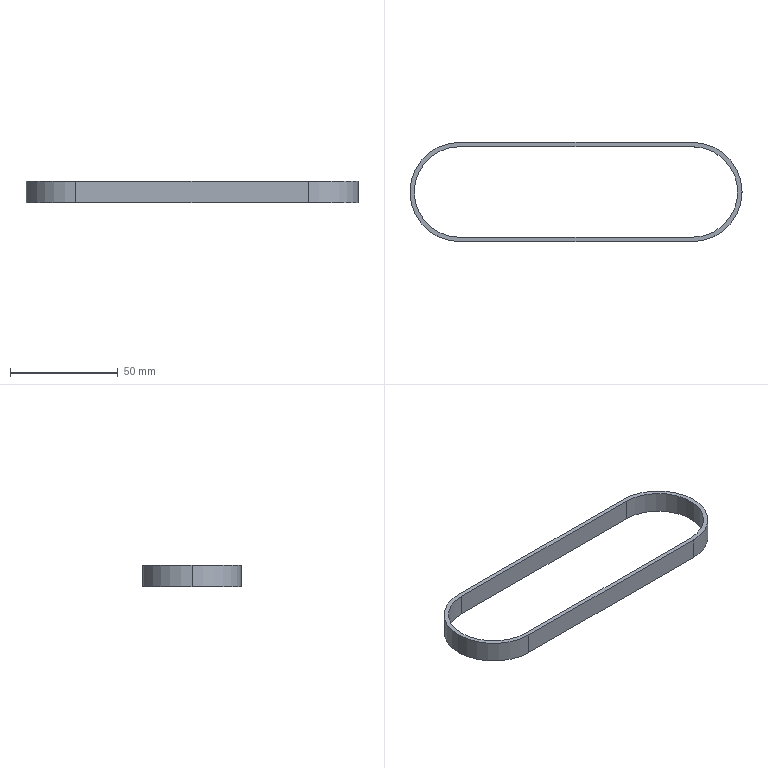Part | SolidWorks | features ExtruThin 1 | 1 solid | 12 faces | box 154 x 46 x 10 mm | volume 7085 mm3 | cylinder 6 | plane 6 | commonest cylinder face diameters 42 x3 46 x3
STEP:
#1=CARTESIAN_POINT('',(0.,21.,5.));
#2=VERTEX_POINT('',#1);
#3=CARTESIAN_POINT('',(-21.,0.,5.));
#4=VERTEX_POINT('',#3);
#5=CARTESIAN_POINT('',(0.,0.,5.));
#6=DIRECTION('',(0.,0.,1.));
#7=DIRECTION('',(1.,0.,0.));
#8=AXIS2_PLACEMENT_3D('',#5,#6,#7);
#9=CIRCLE('',#8,21.);
#10=EDGE_CURVE('',#2,#4,#9,.T.);
#11=ORIENTED_EDGE('',*,*,#10,.T.);
#12=CARTESIAN_POINT('',(-21.,0.,-5.));
#13=VERTEX_POINT('',#12);
#14=CARTESIAN_POINT('',(-21.,0.,5.));
#15=DIRECTION('',(0.,0.,-1.));
#16=VECTOR('',#15,1000.);
#17=LINE('',#14,#16);
#18=EDGE_CURVE('',#4,#13,#17,.T.);
#19=ORIENTED_EDGE('',*,*,#18,.T.);
#20=CARTESIAN_POINT('',(0.,21.,-5.));
#21=VERTEX_POINT('',#20);
#22=CARTESIAN_POINT('',(0.,0.,-5.));
#23=DIRECTION('',(0.,0.,1.));
#24=DIRECTION('',(1.,0.,0.));
#25=AXIS2_PLACEMENT_3D('',#22,#23,#24);
#26=CIRCLE('',#25,21.);
#27=EDGE_CURVE('',#21,#13,#26,.T.);
#28=ORIENTED_EDGE('',*,*,#27,.F.);
#29=CARTESIAN_POINT('',(0.,21.,5.));
#30=DIRECTION('',(0.,0.,-1.));
#31=VECTOR('',#30,1000.);
#32=LINE('',#29,#31);
#33=EDGE_CURVE('',#2,#21,#32,.T.);
#34=ORIENTED_EDGE('',*,*,#33,.F.);
#35=EDGE_LOOP('',(#11,#19,#28,#34));
#36=FACE_OUTER_BOUND('',#35,.T.);
#37=CARTESIAN_POINT('',(0.,0.,5.));
#38=DIRECTION('',(0.,0.,-1.));
#39=DIRECTION('',(-1.,0.,0.));
#40=AXIS2_PLACEMENT_3D('',#37,#38,#39);
#41=CYLINDRICAL_SURFACE('',#40,21.);
#42=ADVANCED_FACE('',(#36),#41,.F.);
#43=CARTESIAN_POINT('',(-23.,0.,5.));
#44=VERTEX_POINT('',#43);
#45=CARTESIAN_POINT('',(0.,-23.,5.));
#46=VERTEX_POINT('',#45);
#47=CARTESIAN_POINT('',(0.,0.,5.));
#48=DIRECTION('',(0.,0.,1.));
#49=DIRECTION('',(1.,0.,0.));
#50=AXIS2_PLACEMENT_3D('',#47,#48,#49);
#51=CIRCLE('',#50,23.);
#52=EDGE_CURVE('',#44,#46,#51,.T.);
#53=ORIENTED_EDGE('',*,*,#52,.F.);
#54=CARTESIAN_POINT('',(-23.,0.,-5.));
#55=VERTEX_POINT('',#54);
#56=CARTESIAN_POINT('',(-23.,0.,5.));
#57=DIRECTION('',(0.,0.,-1.));
#58=VECTOR('',#57,1000.);
#59=LINE('',#56,#58);
#60=EDGE_CURVE('',#44,#55,#59,.T.);
#61=ORIENTED_EDGE('',*,*,#60,.T.);
#62=CARTESIAN_POINT('',(0.,-23.,-5.));
#63=VERTEX_POINT('',#62);
#64=CARTESIAN_POINT('',(0.,0.,-5.));
#65=DIRECTION('',(0.,0.,1.));
#66=DIRECTION('',(1.,0.,0.));
#67=AXIS2_PLACEMENT_3D('',#64,#65,#66);
#68=CIRCLE('',#67,23.);
#69=EDGE_CURVE('',#55,#63,#68,.T.);
#70=ORIENTED_EDGE('',*,*,#69,.T.);
#71=CARTESIAN_POINT('',(0.,-23.,5.));
#72=DIRECTION('',(0.,0.,-1.));
#73=VECTOR('',#72,1000.);
#74=LINE('',#71,#73);
#75=EDGE_CURVE('',#46,#63,#74,.T.);
#76=ORIENTED_EDGE('',*,*,#75,.F.);
#77=EDGE_LOOP('',(#53,#61,#70,#76));
#78=FACE_OUTER_BOUND('',#77,.T.);
#79=CARTESIAN_POINT('',(0.,0.,5.));
#80=DIRECTION('',(0.,0.,-1.));
#81=DIRECTION('',(-1.,0.,0.));
#82=AXIS2_PLACEMENT_3D('',#79,#80,#81);
#83=CYLINDRICAL_SURFACE('',#82,23.);
#84=ADVANCED_FACE('',(#78),#83,.T.);
#85=CARTESIAN_POINT('',(0.,23.,5.));
#86=VERTEX_POINT('',#85);
#87=CARTESIAN_POINT('',(0.,0.,5.));
#88=DIRECTION('',(0.,0.,1.));
#89=DIRECTION('',(1.,0.,0.));
#90=AXIS2_PLACEMENT_3D('',#87,#88,#89);
#91=CIRCLE('',#90,23.);
#92=EDGE_CURVE('',#86,#44,#91,.T.);
#93=ORIENTED_EDGE('',*,*,#92,.T.);
#94=ORIENTED_EDGE('',*,*,#52,.T.);
#95=CARTESIAN_POINT('',(108.,-23.,5.));
#96=VERTEX_POINT('',#95);
#97=CARTESIAN_POINT('',(0.,-23.,5.));
#98=DIRECTION('',(1.,0.,0.));
#99=VECTOR('',#98,1000.);
#100=LINE('',#97,#99);
#101=EDGE_CURVE('',#46,#96,#100,.T.);
#102=ORIENTED_EDGE('',*,*,#101,.T.);
#103=CARTESIAN_POINT('',(108.,23.,5.));
#104=VERTEX_POINT('',#103);
#105=CARTESIAN_POINT('',(108.,0.,5.));
#106=DIRECTION('',(0.,0.,1.));
#107=DIRECTION('',(1.,0.,0.));
#108=AXIS2_PLACEMENT_3D('',#105,#106,#107);
#109=CIRCLE('',#108,23.);
#110=EDGE_CURVE('',#96,#104,#109,.T.);
#111=ORIENTED_EDGE('',*,*,#110,.T.);
#112=CARTESIAN_POINT('',(0.,23.,5.));
#113=DIRECTION('',(-1.,0.,0.));
#114=VECTOR('',#113,1000.);
#115=LINE('',#112,#114);
#116=EDGE_CURVE('',#104,#86,#115,.T.);
#117=ORIENTED_EDGE('',*,*,#116,.T.);
#118=EDGE_LOOP('',(#93,#94,#102,#111,#117));
#119=FACE_OUTER_BOUND('',#118,.T.);
#120=CARTESIAN_POINT('',(0.,-21.,5.));
#121=VERTEX_POINT('',#120);
#122=CARTESIAN_POINT('',(108.,-21.,5.));
#123=VERTEX_POINT('',#122);
#124=CARTESIAN_POINT('',(0.,-21.,5.));
#125=DIRECTION('',(1.,0.,0.));
#126=VECTOR('',#125,1000.);
#127=LINE('',#124,#126);
#128=EDGE_CURVE('',#121,#123,#127,.T.);
#129=ORIENTED_EDGE('',*,*,#128,.F.);
#130=CARTESIAN_POINT('',(0.,0.,5.));
#131=DIRECTION('',(0.,0.,1.));
#132=DIRECTION('',(1.,0.,0.));
#133=AXIS2_PLACEMENT_3D('',#130,#131,#132);
#134=CIRCLE('',#133,21.);
#135=EDGE_CURVE('',#4,#121,#134,.T.);
#136=ORIENTED_EDGE('',*,*,#135,.F.);
#137=ORIENTED_EDGE('',*,*,#10,.F.);
#138=CARTESIAN_POINT('',(108.,21.,5.));
#139=VERTEX_POINT('',#138);
#140=CARTESIAN_POINT('',(0.,21.,5.));
#141=DIRECTION('',(-1.,0.,0.));
#142=VECTOR('',#141,1000.);
#143=LINE('',#140,#142);
#144=EDGE_CURVE('',#139,#2,#143,.T.);
#145=ORIENTED_EDGE('',*,*,#144,.F.);
#146=CARTESIAN_POINT('',(108.,0.,5.));
#147=DIRECTION('',(0.,0.,1.));
#148=DIRECTION('',(1.,0.,0.));
#149=AXIS2_PLACEMENT_3D('',#146,#147,#148);
#150=CIRCLE('',#149,21.);
#151=EDGE_CURVE('',#123,#139,#150,.T.);
#152=ORIENTED_EDGE('',*,*,#151,.F.);
#153=EDGE_LOOP('',(#129,#136,#137,#145,#152));
#154=FACE_BOUND('',#153,.T.);
#155=CARTESIAN_POINT('',(0.,0.,5.));
#156=DIRECTION('',(0.,0.,1.));
#157=DIRECTION('',(1.,0.,0.));
#158=AXIS2_PLACEMENT_3D('',#155,#156,#157);
#159=PLANE('',#158);
#160=ADVANCED_FACE('',(#119,#154),#159,.T.);
#161=CARTESIAN_POINT('',(0.,23.,-5.));
#162=VERTEX_POINT('',#161);
#163=CARTESIAN_POINT('',(0.,0.,-5.));
#164=DIRECTION('',(0.,0.,1.));
#165=DIRECTION('',(1.,0.,0.));
#166=AXIS2_PLACEMENT_3D('',#163,#164,#165);
#167=CIRCLE('',#166,23.);
#168=EDGE_CURVE('',#162,#55,#167,.T.);
#169=ORIENTED_EDGE('',*,*,#168,.F.);
#170=CARTESIAN_POINT('',(108.,23.,-5.));
#171=VERTEX_POINT('',#170);
#172=CARTESIAN_POINT('',(0.,23.,-5.));
#173=DIRECTION('',(-1.,0.,0.));
#174=VECTOR('',#173,1000.);
#175=LINE('',#172,#174);
#176=EDGE_CURVE('',#171,#162,#175,.T.);
#177=ORIENTED_EDGE('',*,*,#176,.F.);
#178=CARTESIAN_POINT('',(108.,-23.,-5.));
#179=VERTEX_POINT('',#178);
#180=CARTESIAN_POINT('',(108.,0.,-5.));
#181=DIRECTION('',(0.,0.,1.));
#182=DIRECTION('',(1.,0.,0.));
#183=AXIS2_PLACEMENT_3D('',#180,#181,#182);
#184=CIRCLE('',#183,23.);
#185=EDGE_CURVE('',#179,#171,#184,.T.);
#186=ORIENTED_EDGE('',*,*,#185,.F.);
#187=CARTESIAN_POINT('',(0.,-23.,-5.));
#188=DIRECTION('',(1.,0.,0.));
#189=VECTOR('',#188,1000.);
#190=LINE('',#187,#189);
#191=EDGE_CURVE('',#63,#179,#190,.T.);
#192=ORIENTED_EDGE('',*,*,#191,.F.);
#193=ORIENTED_EDGE('',*,*,#69,.F.);
#194=EDGE_LOOP('',(#169,#177,#186,#192,#193));
#195=FACE_OUTER_BOUND('',#194,.T.);
#196=ORIENTED_EDGE('',*,*,#27,.T.);
#197=CARTESIAN_POINT('',(0.,-21.,-5.));
#198=VERTEX_POINT('',#197);
#199=CARTESIAN_POINT('',(0.,0.,-5.));
#200=DIRECTION('',(0.,0.,1.));
#201=DIRECTION('',(1.,0.,0.));
#202=AXIS2_PLACEMENT_3D('',#199,#200,#201);
#203=CIRCLE('',#202,21.);
#204=EDGE_CURVE('',#13,#198,#203,.T.);
#205=ORIENTED_EDGE('',*,*,#204,.T.);
#206=CARTESIAN_POINT('',(108.,-21.,-5.));
#207=VERTEX_POINT('',#206);
#208=CARTESIAN_POINT('',(0.,-21.,-5.));
#209=DIRECTION('',(1.,0.,0.));
#210=VECTOR('',#209,1000.);
#211=LINE('',#208,#210);
#212=EDGE_CURVE('',#198,#207,#211,.T.);
#213=ORIENTED_EDGE('',*,*,#212,.T.);
#214=CARTESIAN_POINT('',(108.,21.,-5.));
#215=VERTEX_POINT('',#214);
#216=CARTESIAN_POINT('',(108.,0.,-5.));
#217=DIRECTION('',(0.,0.,1.));
#218=DIRECTION('',(1.,0.,0.));
#219=AXIS2_PLACEMENT_3D('',#216,#217,#218);
#220=CIRCLE('',#219,21.);
#221=EDGE_CURVE('',#207,#215,#220,.T.);
#222=ORIENTED_EDGE('',*,*,#221,.T.);
#223=CARTESIAN_POINT('',(0.,21.,-5.));
#224=DIRECTION('',(-1.,0.,0.));
#225=VECTOR('',#224,1000.);
#226=LINE('',#223,#225);
#227=EDGE_CURVE('',#215,#21,#226,.T.);
#228=ORIENTED_EDGE('',*,*,#227,.T.);
#229=EDGE_LOOP('',(#196,#205,#213,#222,#228));
#230=FACE_BOUND('',#229,.T.);
#231=CARTESIAN_POINT('',(0.,0.,-5.));
#232=DIRECTION('',(0.,0.,1.));
#233=DIRECTION('',(1.,0.,0.));
#234=AXIS2_PLACEMENT_3D('',#231,#232,#233);
#235=PLANE('',#234);
#236=ADVANCED_FACE('',(#195,#230),#235,.F.);
#237=ORIENTED_EDGE('',*,*,#60,.F.);
#238=ORIENTED_EDGE('',*,*,#92,.F.);
#239=CARTESIAN_POINT('',(0.,23.,5.));
#240=DIRECTION('',(0.,0.,-1.));
#241=VECTOR('',#240,1000.);
#242=LINE('',#239,#241);
#243=EDGE_CURVE('',#86,#162,#242,.T.);
#244=ORIENTED_EDGE('',*,*,#243,.T.);
#245=ORIENTED_EDGE('',*,*,#168,.T.);
#246=EDGE_LOOP('',(#237,#238,#244,#245));
#247=FACE_OUTER_BOUND('',#246,.T.);
#248=CARTESIAN_POINT('',(0.,0.,5.));
#249=DIRECTION('',(0.,0.,-1.));
#250=DIRECTION('',(-1.,0.,0.));
#251=AXIS2_PLACEMENT_3D('',#248,#249,#250);
#252=CYLINDRICAL_SURFACE('',#251,23.);
#253=ADVANCED_FACE('',(#247),#252,.T.);
#254=ORIENTED_EDGE('',*,*,#191,.T.);
#255=CARTESIAN_POINT('',(108.,-23.,5.));
#256=DIRECTION('',(0.,0.,-1.));
#257=VECTOR('',#256,1000.);
#258=LINE('',#255,#257);
#259=EDGE_CURVE('',#96,#179,#258,.T.);
#260=ORIENTED_EDGE('',*,*,#259,.F.);
#261=ORIENTED_EDGE('',*,*,#101,.F.);
#262=ORIENTED_EDGE('',*,*,#75,.T.);
#263=EDGE_LOOP('',(#254,#260,#261,#262));
#264=FACE_OUTER_BOUND('',#263,.T.);
#265=CARTESIAN_POINT('',(0.,-23.,5.));
#266=DIRECTION('',(0.,1.,0.));
#267=DIRECTION('',(0.,0.,1.));
#268=AXIS2_PLACEMENT_3D('',#265,#266,#267);
#269=PLANE('',#268);
#270=ADVANCED_FACE('',(#264),#269,.F.);
#271=ORIENTED_EDGE('',*,*,#185,.T.);
#272=CARTESIAN_POINT('',(108.,23.,5.));
#273=DIRECTION('',(0.,0.,-1.));
#274=VECTOR('',#273,1000.);
#275=LINE('',#272,#274);
#276=EDGE_CURVE('',#104,#171,#275,.T.);
#277=ORIENTED_EDGE('',*,*,#276,.F.);
#278=ORIENTED_EDGE('',*,*,#110,.F.);
#279=ORIENTED_EDGE('',*,*,#259,.T.);
#280=EDGE_LOOP('',(#271,#277,#278,#279));
#281=FACE_OUTER_BOUND('',#280,.T.);
#282=CARTESIAN_POINT('',(108.,0.,5.));
#283=DIRECTION('',(0.,0.,-1.));
#284=DIRECTION('',(-1.,0.,0.));
#285=AXIS2_PLACEMENT_3D('',#282,#283,#284);
#286=CYLINDRICAL_SURFACE('',#285,23.);
#287=ADVANCED_FACE('',(#281),#286,.T.);
#288=ORIENTED_EDGE('',*,*,#176,.T.);
#289=ORIENTED_EDGE('',*,*,#243,.F.);
#290=ORIENTED_EDGE('',*,*,#116,.F.);
#291=ORIENTED_EDGE('',*,*,#276,.T.);
#292=EDGE_LOOP('',(#288,#289,#290,#291));
#293=FACE_OUTER_BOUND('',#292,.T.);
#294=CARTESIAN_POINT('',(0.,23.,5.));
#295=DIRECTION('',(0.,-1.,0.));
#296=DIRECTION('',(0.,0.,-1.));
#297=AXIS2_PLACEMENT_3D('',#294,#295,#296);
#298=PLANE('',#297);
#299=ADVANCED_FACE('',(#293),#298,.F.);
#300=ORIENTED_EDGE('',*,*,#18,.F.);
#301=ORIENTED_EDGE('',*,*,#135,.T.);
#302=CARTESIAN_POINT('',(0.,-21.,5.));
#303=DIRECTION('',(0.,0.,-1.));
#304=VECTOR('',#303,1000.);
#305=LINE('',#302,#304);
#306=EDGE_CURVE('',#121,#198,#305,.T.);
#307=ORIENTED_EDGE('',*,*,#306,.T.);
#308=ORIENTED_EDGE('',*,*,#204,.F.);
#309=EDGE_LOOP('',(#300,#301,#307,#308));
#310=FACE_OUTER_BOUND('',#309,.T.);
#311=CARTESIAN_POINT('',(0.,0.,5.));
#312=DIRECTION('',(0.,0.,-1.));
#313=DIRECTION('',(-1.,0.,0.));
#314=AXIS2_PLACEMENT_3D('',#311,#312,#313);
#315=CYLINDRICAL_SURFACE('',#314,21.);
#316=ADVANCED_FACE('',(#310),#315,.F.);
#317=ORIENTED_EDGE('',*,*,#212,.F.);
#318=ORIENTED_EDGE('',*,*,#306,.F.);
#319=ORIENTED_EDGE('',*,*,#128,.T.);
#320=CARTESIAN_POINT('',(108.,-21.,5.));
#321=DIRECTION('',(0.,0.,-1.));
#322=VECTOR('',#321,1000.);
#323=LINE('',#320,#322);
#324=EDGE_CURVE('',#123,#207,#323,.T.);
#325=ORIENTED_EDGE('',*,*,#324,.T.);
#326=EDGE_LOOP('',(#317,#318,#319,#325));
#327=FACE_OUTER_BOUND('',#326,.T.);
#328=CARTESIAN_POINT('',(0.,-21.,5.));
#329=DIRECTION('',(0.,1.,0.));
#330=DIRECTION('',(0.,0.,1.));
#331=AXIS2_PLACEMENT_3D('',#328,#329,#330);
#332=PLANE('',#331);
#333=ADVANCED_FACE('',(#327),#332,.T.);
#334=ORIENTED_EDGE('',*,*,#221,.F.);
#335=ORIENTED_EDGE('',*,*,#324,.F.);
#336=ORIENTED_EDGE('',*,*,#151,.T.);
#337=CARTESIAN_POINT('',(108.,21.,5.));
#338=DIRECTION('',(0.,0.,-1.));
#339=VECTOR('',#338,1000.);
#340=LINE('',#337,#339);
#341=EDGE_CURVE('',#139,#215,#340,.T.);
#342=ORIENTED_EDGE('',*,*,#341,.T.);
#343=EDGE_LOOP('',(#334,#335,#336,#342));
#344=FACE_OUTER_BOUND('',#343,.T.);
#345=CARTESIAN_POINT('',(108.,0.,5.));
#346=DIRECTION('',(0.,0.,-1.));
#347=DIRECTION('',(-1.,0.,0.));
#348=AXIS2_PLACEMENT_3D('',#345,#346,#347);
#349=CYLINDRICAL_SURFACE('',#348,21.);
#350=ADVANCED_FACE('',(#344),#349,.F.);
#351=ORIENTED_EDGE('',*,*,#227,.F.);
#352=ORIENTED_EDGE('',*,*,#341,.F.);
#353=ORIENTED_EDGE('',*,*,#144,.T.);
#354=ORIENTED_EDGE('',*,*,#33,.T.);
#355=EDGE_LOOP('',(#351,#352,#353,#354));
#356=FACE_OUTER_BOUND('',#355,.T.);
#357=CARTESIAN_POINT('',(0.,21.,5.));
#358=DIRECTION('',(0.,-1.,0.));
#359=DIRECTION('',(0.,0.,-1.));
#360=AXIS2_PLACEMENT_3D('',#357,#358,#359);
#361=PLANE('',#360);
#362=ADVANCED_FACE('',(#356),#361,.T.);
#363=CLOSED_SHELL('',(#42,#84,#160,#236,#253,#270,#287,#299,#316,#333,#350,#362));
#364=MANIFOLD_SOLID_BREP('',#363);
#365=CARTESIAN_POINT('',(0.,0.,0.));
#366=DIRECTION('',(0.,0.,1.));
#367=DIRECTION('',(1.,0.,0.));
#368=AXIS2_PLACEMENT_3D('',#365,#366,#367);
#369=(LENGTH_UNIT()NAMED_UNIT(*)SI_UNIT(.MILLI.,.METRE.));
#370=UNCERTAINTY_MEASURE_WITH_UNIT(LENGTH_MEASURE(0.00001),#369,'','');
#371=(NAMED_UNIT(*)PLANE_ANGLE_UNIT()SI_UNIT($,.RADIAN.));
#372=(NAMED_UNIT(*)SI_UNIT($,.STERADIAN.)SOLID_ANGLE_UNIT());
#373=(GEOMETRIC_REPRESENTATION_CONTEXT(3)GLOBAL_UNCERTAINTY_ASSIGNED_CONTEXT((#370))GLOBAL_UNIT_ASSIGNED_CONTEXT((#369,#371,#372))REPRESENTATION_CONTEXT('',''));
#374=ADVANCED_BREP_SHAPE_REPRESENTATION('',(#364,#368),#373);